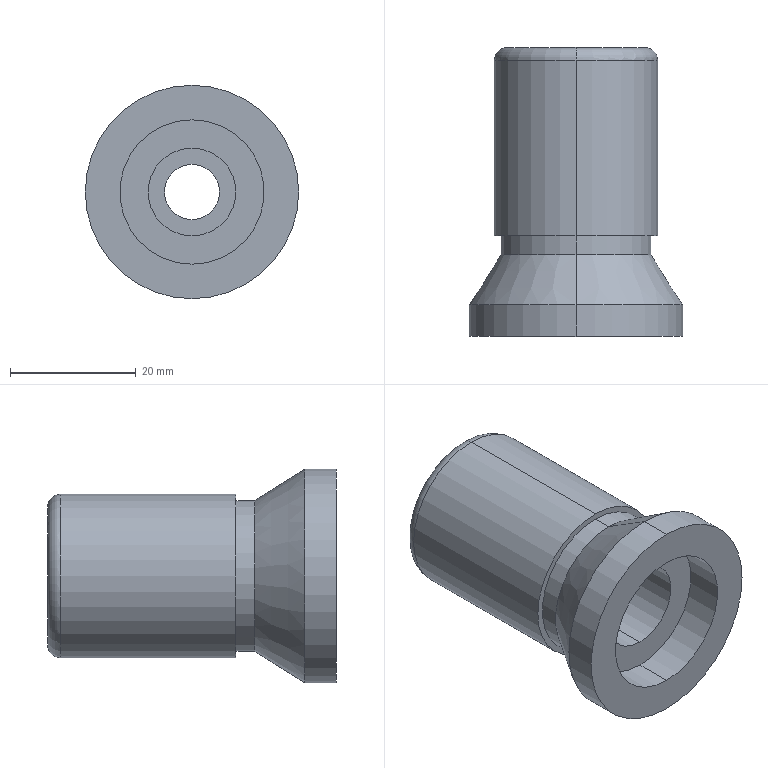Part | STEP file | 刮-墨刀压力镙母-1 | 1 solid | 21 faces | box 34 x 46 x 34 mm | volume 20305 mm3 | cylinder 12 | plane 5 | torus 2 | cone 2 | commonest cylinder face diameters 8.8 x2 14 x2 23 x2 24 x2 26 x2 34 x2
STEP:
#1=CARTESIAN_POINT('',(0.,0.,11.));
#2=VERTEX_POINT('',#1);
#3=CARTESIAN_POINT('',(0.,0.,-11.));
#4=VERTEX_POINT('',#3);
#5=CARTESIAN_POINT('',(0.,0.,0.));
#6=DIRECTION('',(0.,1.,0.));
#7=DIRECTION('',(0.,0.,-1.));
#8=AXIS2_PLACEMENT_3D('',#5,#6,#7);
#9=CIRCLE('',#8,11.);
#10=EDGE_CURVE('',#2,#4,#9,.T.);
#11=ORIENTED_EDGE('',*,*,#10,.F.);
#12=CARTESIAN_POINT('',(0.,-2.,13.));
#13=VERTEX_POINT('',#12);
#14=CARTESIAN_POINT('',(0.,-2.,11.));
#15=DIRECTION('',(1.,0.,0.));
#16=DIRECTION('',(0.,0.,-1.));
#17=AXIS2_PLACEMENT_3D('',#14,#15,#16);
#18=CIRCLE('',#17,2.);
#19=EDGE_CURVE('',#2,#13,#18,.T.);
#20=ORIENTED_EDGE('',*,*,#19,.T.);
#21=CARTESIAN_POINT('',(0.,-2.,-13.));
#22=VERTEX_POINT('',#21);
#23=CARTESIAN_POINT('',(0.,-2.,0.));
#24=DIRECTION('',(0.,-1.,0.));
#25=DIRECTION('',(0.,0.,-1.));
#26=AXIS2_PLACEMENT_3D('',#23,#24,#25);
#27=CIRCLE('',#26,13.);
#28=EDGE_CURVE('',#22,#13,#27,.T.);
#29=ORIENTED_EDGE('',*,*,#28,.F.);
#30=CARTESIAN_POINT('',(0.,-2.,-11.));
#31=DIRECTION('',(-1.,0.,0.));
#32=DIRECTION('',(0.,0.,1.));
#33=AXIS2_PLACEMENT_3D('',#30,#31,#32);
#34=CIRCLE('',#33,2.);
#35=EDGE_CURVE('',#4,#22,#34,.T.);
#36=ORIENTED_EDGE('',*,*,#35,.F.);
#37=EDGE_LOOP('',(#11,#20,#29,#36));
#38=FACE_OUTER_BOUND('',#37,.T.);
#39=CARTESIAN_POINT('',(0.,-2.,0.));
#40=DIRECTION('',(0.,-1.,0.));
#41=DIRECTION('',(0.,0.,-1.));
#42=AXIS2_PLACEMENT_3D('',#39,#40,#41);
#43=TOROIDAL_SURFACE('',#42,11.,2.);
#44=ADVANCED_FACE('',(#38),#43,.T.);
#45=CARTESIAN_POINT('',(0.,-20.,4.4));
#46=VERTEX_POINT('',#45);
#47=CARTESIAN_POINT('',(0.,-20.,-4.4));
#48=VERTEX_POINT('',#47);
#49=CARTESIAN_POINT('',(0.,-20.,0.));
#50=DIRECTION('',(0.,-1.,0.));
#51=DIRECTION('',(0.,0.,-1.));
#52=AXIS2_PLACEMENT_3D('',#49,#50,#51);
#53=CIRCLE('',#52,4.4);
#54=EDGE_CURVE('',#46,#48,#53,.T.);
#55=ORIENTED_EDGE('',*,*,#54,.T.);
#56=CARTESIAN_POINT('',(0.,0.,-4.4));
#57=VERTEX_POINT('',#56);
#58=CARTESIAN_POINT('',(0.,0.,-4.4));
#59=DIRECTION('',(0.,1.,0.));
#60=VECTOR('',#59,1000.);
#61=LINE('',#58,#60);
#62=EDGE_CURVE('',#48,#57,#61,.T.);
#63=ORIENTED_EDGE('',*,*,#62,.T.);
#64=CARTESIAN_POINT('',(0.,0.,4.4));
#65=VERTEX_POINT('',#64);
#66=CARTESIAN_POINT('',(0.,0.,0.));
#67=DIRECTION('',(0.,1.,0.));
#68=DIRECTION('',(0.,0.,1.));
#69=AXIS2_PLACEMENT_3D('',#66,#67,#68);
#70=CIRCLE('',#69,4.4);
#71=EDGE_CURVE('',#57,#65,#70,.T.);
#72=ORIENTED_EDGE('',*,*,#71,.T.);
#73=CARTESIAN_POINT('',(0.,0.,4.4));
#74=DIRECTION('',(0.,1.,0.));
#75=VECTOR('',#74,1000.);
#76=LINE('',#73,#75);
#77=EDGE_CURVE('',#46,#65,#76,.T.);
#78=ORIENTED_EDGE('',*,*,#77,.F.);
#79=EDGE_LOOP('',(#55,#63,#72,#78));
#80=FACE_OUTER_BOUND('',#79,.T.);
#81=CARTESIAN_POINT('',(0.,0.,0.));
#82=DIRECTION('',(0.,1.,0.));
#83=DIRECTION('',(0.,0.,1.));
#84=AXIS2_PLACEMENT_3D('',#81,#82,#83);
#85=CYLINDRICAL_SURFACE('',#84,4.4);
#86=ADVANCED_FACE('',(#80),#85,.F.);
#87=CARTESIAN_POINT('',(0.,-20.,7.));
#88=VERTEX_POINT('',#87);
#89=CARTESIAN_POINT('',(0.,-20.,-7.));
#90=VERTEX_POINT('',#89);
#91=CARTESIAN_POINT('',(0.,-20.,0.));
#92=DIRECTION('',(0.,-1.,0.));
#93=DIRECTION('',(0.,0.,-1.));
#94=AXIS2_PLACEMENT_3D('',#91,#92,#93);
#95=CIRCLE('',#94,7.);
#96=EDGE_CURVE('',#88,#90,#95,.T.);
#97=ORIENTED_EDGE('',*,*,#96,.F.);
#98=CARTESIAN_POINT('',(0.,-40.,7.));
#99=VERTEX_POINT('',#98);
#100=CARTESIAN_POINT('',(0.,-20.,7.));
#101=DIRECTION('',(0.,-1.,0.));
#102=VECTOR('',#101,1000.);
#103=LINE('',#100,#102);
#104=EDGE_CURVE('',#88,#99,#103,.T.);
#105=ORIENTED_EDGE('',*,*,#104,.T.);
#106=CARTESIAN_POINT('',(0.,-40.,-7.));
#107=VERTEX_POINT('',#106);
#108=CARTESIAN_POINT('',(0.,-40.,0.));
#109=DIRECTION('',(0.,-1.,0.));
#110=DIRECTION('',(0.,0.,-1.));
#111=AXIS2_PLACEMENT_3D('',#108,#109,#110);
#112=CIRCLE('',#111,7.);
#113=EDGE_CURVE('',#99,#107,#112,.T.);
#114=ORIENTED_EDGE('',*,*,#113,.T.);
#115=CARTESIAN_POINT('',(0.,-20.,-7.));
#116=DIRECTION('',(0.,-1.,0.));
#117=VECTOR('',#116,1000.);
#118=LINE('',#115,#117);
#119=EDGE_CURVE('',#90,#107,#118,.T.);
#120=ORIENTED_EDGE('',*,*,#119,.F.);
#121=EDGE_LOOP('',(#97,#105,#114,#120));
#122=FACE_OUTER_BOUND('',#121,.T.);
#123=CARTESIAN_POINT('',(0.,-20.,0.));
#124=DIRECTION('',(0.,-1.,0.));
#125=DIRECTION('',(0.,0.,-1.));
#126=AXIS2_PLACEMENT_3D('',#123,#124,#125);
#127=CYLINDRICAL_SURFACE('',#126,7.);
#128=ADVANCED_FACE('',(#122),#127,.F.);
#129=CARTESIAN_POINT('',(0.,-40.,11.5));
#130=VERTEX_POINT('',#129);
#131=CARTESIAN_POINT('',(0.,-40.,-11.5));
#132=VERTEX_POINT('',#131);
#133=CARTESIAN_POINT('',(0.,-40.,0.));
#134=DIRECTION('',(0.,-1.,0.));
#135=DIRECTION('',(0.,0.,-1.));
#136=AXIS2_PLACEMENT_3D('',#133,#134,#135);
#137=CIRCLE('',#136,11.5);
#138=EDGE_CURVE('',#130,#132,#137,.T.);
#139=ORIENTED_EDGE('',*,*,#138,.F.);
#140=CARTESIAN_POINT('',(0.,-46.,11.5));
#141=VERTEX_POINT('',#140);
#142=CARTESIAN_POINT('',(0.,-40.,11.5));
#143=DIRECTION('',(0.,-1.,0.));
#144=VECTOR('',#143,1000.);
#145=LINE('',#142,#144);
#146=EDGE_CURVE('',#130,#141,#145,.T.);
#147=ORIENTED_EDGE('',*,*,#146,.T.);
#148=CARTESIAN_POINT('',(0.,-46.,-11.5));
#149=VERTEX_POINT('',#148);
#150=CARTESIAN_POINT('',(0.,-46.,0.));
#151=DIRECTION('',(0.,-1.,0.));
#152=DIRECTION('',(0.,0.,-1.));
#153=AXIS2_PLACEMENT_3D('',#150,#151,#152);
#154=CIRCLE('',#153,11.5);
#155=EDGE_CURVE('',#141,#149,#154,.T.);
#156=ORIENTED_EDGE('',*,*,#155,.T.);
#157=CARTESIAN_POINT('',(0.,-40.,-11.5));
#158=DIRECTION('',(0.,-1.,0.));
#159=VECTOR('',#158,1000.);
#160=LINE('',#157,#159);
#161=EDGE_CURVE('',#132,#149,#160,.T.);
#162=ORIENTED_EDGE('',*,*,#161,.F.);
#163=EDGE_LOOP('',(#139,#147,#156,#162));
#164=FACE_OUTER_BOUND('',#163,.T.);
#165=CARTESIAN_POINT('',(0.,-40.,0.));
#166=DIRECTION('',(0.,-1.,0.));
#167=DIRECTION('',(0.,0.,-1.));
#168=AXIS2_PLACEMENT_3D('',#165,#166,#167);
#169=CYLINDRICAL_SURFACE('',#168,11.5);
#170=ADVANCED_FACE('',(#164),#169,.F.);
#171=CARTESIAN_POINT('',(0.,-46.,17.));
#172=VERTEX_POINT('',#171);
#173=CARTESIAN_POINT('',(0.,-46.,-17.));
#174=VERTEX_POINT('',#173);
#175=CARTESIAN_POINT('',(0.,-46.,0.));
#176=DIRECTION('',(0.,1.,0.));
#177=DIRECTION('',(0.,0.,1.));
#178=AXIS2_PLACEMENT_3D('',#175,#176,#177);
#179=CIRCLE('',#178,17.);
#180=EDGE_CURVE('',#172,#174,#179,.T.);
#181=ORIENTED_EDGE('',*,*,#180,.T.);
#182=CARTESIAN_POINT('',(0.,-41.,-17.));
#183=VERTEX_POINT('',#182);
#184=CARTESIAN_POINT('',(0.,0.,-17.));
#185=DIRECTION('',(0.,1.,0.));
#186=VECTOR('',#185,1000.);
#187=LINE('',#184,#186);
#188=EDGE_CURVE('',#174,#183,#187,.T.);
#189=ORIENTED_EDGE('',*,*,#188,.T.);
#190=CARTESIAN_POINT('',(0.,-41.,17.));
#191=VERTEX_POINT('',#190);
#192=CARTESIAN_POINT('',(0.,-41.,0.));
#193=DIRECTION('',(0.,1.,0.));
#194=DIRECTION('',(0.,0.,1.));
#195=AXIS2_PLACEMENT_3D('',#192,#193,#194);
#196=CIRCLE('',#195,17.);
#197=EDGE_CURVE('',#191,#183,#196,.T.);
#198=ORIENTED_EDGE('',*,*,#197,.F.);
#199=CARTESIAN_POINT('',(0.,0.,17.));
#200=DIRECTION('',(0.,1.,0.));
#201=VECTOR('',#200,1000.);
#202=LINE('',#199,#201);
#203=EDGE_CURVE('',#172,#191,#202,.T.);
#204=ORIENTED_EDGE('',*,*,#203,.F.);
#205=EDGE_LOOP('',(#181,#189,#198,#204));
#206=FACE_OUTER_BOUND('',#205,.T.);
#207=CARTESIAN_POINT('',(0.,0.,0.));
#208=DIRECTION('',(0.,1.,0.));
#209=DIRECTION('',(0.,0.,1.));
#210=AXIS2_PLACEMENT_3D('',#207,#208,#209);
#211=CYLINDRICAL_SURFACE('',#210,17.);
#212=ADVANCED_FACE('',(#206),#211,.T.);
#213=CARTESIAN_POINT('',(0.,-33.,12.));
#214=VERTEX_POINT('',#213);
#215=CARTESIAN_POINT('',(0.,-33.,-12.));
#216=VERTEX_POINT('',#215);
#217=CARTESIAN_POINT('',(0.,-33.,0.));
#218=DIRECTION('',(0.,1.,0.));
#219=DIRECTION('',(0.,0.,1.));
#220=AXIS2_PLACEMENT_3D('',#217,#218,#219);
#221=CIRCLE('',#220,12.);
#222=EDGE_CURVE('',#214,#216,#221,.T.);
#223=ORIENTED_EDGE('',*,*,#222,.F.);
#224=CARTESIAN_POINT('',(0.,-41.,17.));
#225=DIRECTION('',(0.,-0.848,0.53));
#226=VECTOR('',#225,1000.);
#227=LINE('',#224,#226);
#228=EDGE_CURVE('',#214,#191,#227,.T.);
#229=ORIENTED_EDGE('',*,*,#228,.T.);
#230=ORIENTED_EDGE('',*,*,#197,.T.);
#231=CARTESIAN_POINT('',(0.,-41.,-17.));
#232=DIRECTION('',(0.,-0.848,-0.53));
#233=VECTOR('',#232,1000.);
#234=LINE('',#231,#233);
#235=EDGE_CURVE('',#216,#183,#234,.T.);
#236=ORIENTED_EDGE('',*,*,#235,.F.);
#237=EDGE_LOOP('',(#223,#229,#230,#236));
#238=FACE_OUTER_BOUND('',#237,.T.);
#239=CARTESIAN_POINT('',(0.,-41.,0.));
#240=DIRECTION('',(0.,-1.,0.));
#241=DIRECTION('',(0.,0.,-1.));
#242=AXIS2_PLACEMENT_3D('',#239,#240,#241);
#243=CONICAL_SURFACE('',#242,17.,0.5586);
#244=ADVANCED_FACE('',(#238),#243,.T.);
#245=ORIENTED_EDGE('',*,*,#222,.T.);
#246=CARTESIAN_POINT('',(0.,-30.,-12.));
#247=VERTEX_POINT('',#246);
#248=CARTESIAN_POINT('',(0.,0.,-12.));
#249=DIRECTION('',(0.,1.,0.));
#250=VECTOR('',#249,1000.);
#251=LINE('',#248,#250);
#252=EDGE_CURVE('',#216,#247,#251,.T.);
#253=ORIENTED_EDGE('',*,*,#252,.T.);
#254=CARTESIAN_POINT('',(0.,-30.,12.));
#255=VERTEX_POINT('',#254);
#256=CARTESIAN_POINT('',(0.,-30.,0.));
#257=DIRECTION('',(0.,1.,0.));
#258=DIRECTION('',(0.,0.,1.));
#259=AXIS2_PLACEMENT_3D('',#256,#257,#258);
#260=CIRCLE('',#259,12.);
#261=EDGE_CURVE('',#255,#247,#260,.T.);
#262=ORIENTED_EDGE('',*,*,#261,.F.);
#263=CARTESIAN_POINT('',(0.,0.,12.));
#264=DIRECTION('',(0.,1.,0.));
#265=VECTOR('',#264,1000.);
#266=LINE('',#263,#265);
#267=EDGE_CURVE('',#214,#255,#266,.T.);
#268=ORIENTED_EDGE('',*,*,#267,.F.);
#269=EDGE_LOOP('',(#245,#253,#262,#268));
#270=FACE_OUTER_BOUND('',#269,.T.);
#271=CARTESIAN_POINT('',(0.,0.,0.));
#272=DIRECTION('',(0.,1.,0.));
#273=DIRECTION('',(0.,0.,1.));
#274=AXIS2_PLACEMENT_3D('',#271,#272,#273);
#275=CYLINDRICAL_SURFACE('',#274,12.);
#276=ADVANCED_FACE('',(#270),#275,.T.);
#277=CARTESIAN_POINT('',(0.,-30.,13.));
#278=VERTEX_POINT('',#277);
#279=CARTESIAN_POINT('',(0.,-30.,-13.));
#280=VERTEX_POINT('',#279);
#281=CARTESIAN_POINT('',(0.,-30.,0.));
#282=DIRECTION('',(0.,1.,0.));
#283=DIRECTION('',(0.,0.,1.));
#284=AXIS2_PLACEMENT_3D('',#281,#282,#283);
#285=CIRCLE('',#284,13.);
#286=EDGE_CURVE('',#278,#280,#285,.T.);
#287=ORIENTED_EDGE('',*,*,#286,.T.);
#288=CARTESIAN_POINT('',(0.,0.,-13.));
#289=DIRECTION('',(0.,1.,0.));
#290=VECTOR('',#289,1000.);
#291=LINE('',#288,#290);
#292=EDGE_CURVE('',#280,#22,#291,.T.);
#293=ORIENTED_EDGE('',*,*,#292,.T.);
#294=ORIENTED_EDGE('',*,*,#28,.T.);
#295=CARTESIAN_POINT('',(0.,0.,13.));
#296=DIRECTION('',(0.,1.,0.));
#297=VECTOR('',#296,1000.);
#298=LINE('',#295,#297);
#299=EDGE_CURVE('',#278,#13,#298,.T.);
#300=ORIENTED_EDGE('',*,*,#299,.F.);
#301=EDGE_LOOP('',(#287,#293,#294,#300));
#302=FACE_OUTER_BOUND('',#301,.T.);
#303=CARTESIAN_POINT('',(0.,0.,0.));
#304=DIRECTION('',(0.,1.,0.));
#305=DIRECTION('',(0.,0.,1.));
#306=AXIS2_PLACEMENT_3D('',#303,#304,#305);
#307=CYLINDRICAL_SURFACE('',#306,13.);
#308=ADVANCED_FACE('',(#302),#307,.T.);
#309=CARTESIAN_POINT('',(0.,0.,0.));
#310=DIRECTION('',(0.,1.,0.));
#311=DIRECTION('',(0.,0.,-1.));
#312=AXIS2_PLACEMENT_3D('',#309,#310,#311);
#313=CIRCLE('',#312,11.);
#314=EDGE_CURVE('',#4,#2,#313,.T.);
#315=ORIENTED_EDGE('',*,*,#314,.T.);
#316=ORIENTED_EDGE('',*,*,#10,.T.);
#317=EDGE_LOOP('',(#315,#316));
#318=FACE_OUTER_BOUND('',#317,.T.);
#319=CARTESIAN_POINT('',(0.,0.,0.));
#320=DIRECTION('',(0.,1.,0.));
#321=DIRECTION('',(0.,0.,1.));
#322=AXIS2_PLACEMENT_3D('',#319,#320,#321);
#323=CIRCLE('',#322,4.4);
#324=EDGE_CURVE('',#65,#57,#323,.T.);
#325=ORIENTED_EDGE('',*,*,#324,.F.);
#326=ORIENTED_EDGE('',*,*,#71,.F.);
#327=EDGE_LOOP('',(#325,#326));
#328=FACE_BOUND('',#327,.T.);
#329=CARTESIAN_POINT('',(0.,0.,0.));
#330=DIRECTION('',(0.,-1.,0.));
#331=DIRECTION('',(0.,0.,-1.));
#332=AXIS2_PLACEMENT_3D('',#329,#330,#331);
#333=PLANE('',#332);
#334=ADVANCED_FACE('',(#318,#328),#333,.F.);
#335=ORIENTED_EDGE('',*,*,#292,.F.);
#336=CARTESIAN_POINT('',(0.,-30.,0.));
#337=DIRECTION('',(0.,1.,0.));
#338=DIRECTION('',(0.,0.,1.));
#339=AXIS2_PLACEMENT_3D('',#336,#337,#338);
#340=CIRCLE('',#339,13.);
#341=EDGE_CURVE('',#280,#278,#340,.T.);
#342=ORIENTED_EDGE('',*,*,#341,.T.);
#343=ORIENTED_EDGE('',*,*,#299,.T.);
#344=CARTESIAN_POINT('',(0.,-2.,0.));
#345=DIRECTION('',(0.,-1.,0.));
#346=DIRECTION('',(0.,0.,-1.));
#347=AXIS2_PLACEMENT_3D('',#344,#345,#346);
#348=CIRCLE('',#347,13.);
#349=EDGE_CURVE('',#13,#22,#348,.T.);
#350=ORIENTED_EDGE('',*,*,#349,.T.);
#351=EDGE_LOOP('',(#335,#342,#343,#350));
#352=FACE_OUTER_BOUND('',#351,.T.);
#353=CARTESIAN_POINT('',(0.,0.,0.));
#354=DIRECTION('',(0.,1.,0.));
#355=DIRECTION('',(0.,0.,1.));
#356=AXIS2_PLACEMENT_3D('',#353,#354,#355);
#357=CYLINDRICAL_SURFACE('',#356,13.);
#358=ADVANCED_FACE('',(#352),#357,.T.);
#359=ORIENTED_EDGE('',*,*,#286,.F.);
#360=ORIENTED_EDGE('',*,*,#341,.F.);
#361=EDGE_LOOP('',(#359,#360));
#362=FACE_OUTER_BOUND('',#361,.T.);
#363=ORIENTED_EDGE('',*,*,#261,.T.);
#364=CARTESIAN_POINT('',(0.,-30.,0.));
#365=DIRECTION('',(0.,1.,0.));
#366=DIRECTION('',(0.,0.,1.));
#367=AXIS2_PLACEMENT_3D('',#364,#365,#366);
#368=CIRCLE('',#367,12.);
#369=EDGE_CURVE('',#247,#255,#368,.T.);
#370=ORIENTED_EDGE('',*,*,#369,.T.);
#371=EDGE_LOOP('',(#363,#370));
#372=FACE_BOUND('',#371,.T.);
#373=CARTESIAN_POINT('',(13.,-30.,0.));
#374=DIRECTION('',(0.,1.,0.));
#375=DIRECTION('',(0.,0.,1.));
#376=AXIS2_PLACEMENT_3D('',#373,#374,#375);
#377=PLANE('',#376);
#378=ADVANCED_FACE('',(#362,#372),#377,.F.);
#379=ORIENTED_EDGE('',*,*,#252,.F.);
#380=CARTESIAN_POINT('',(0.,-33.,0.));
#381=DIRECTION('',(0.,1.,0.));
#382=DIRECTION('',(0.,0.,1.));
#383=AXIS2_PLACEMENT_3D('',#380,#381,#382);
#384=CIRCLE('',#383,12.);
#385=EDGE_CURVE('',#216,#214,#384,.T.);
#386=ORIENTED_EDGE('',*,*,#385,.T.);
#387=ORIENTED_EDGE('',*,*,#267,.T.);
#388=ORIENTED_EDGE('',*,*,#369,.F.);
#389=EDGE_LOOP('',(#379,#386,#387,#388));
#390=FACE_OUTER_BOUND('',#389,.T.);
#391=CARTESIAN_POINT('',(0.,0.,0.));
#392=DIRECTION('',(0.,1.,0.));
#393=DIRECTION('',(0.,0.,1.));
#394=AXIS2_PLACEMENT_3D('',#391,#392,#393);
#395=CYLINDRICAL_SURFACE('',#394,12.);
#396=ADVANCED_FACE('',(#390),#395,.T.);
#397=ORIENTED_EDGE('',*,*,#228,.F.);
#398=ORIENTED_EDGE('',*,*,#385,.F.);
#399=ORIENTED_EDGE('',*,*,#235,.T.);
#400=CARTESIAN_POINT('',(0.,-41.,0.));
#401=DIRECTION('',(0.,1.,0.));
#402=DIRECTION('',(0.,0.,1.));
#403=AXIS2_PLACEMENT_3D('',#400,#401,#402);
#404=CIRCLE('',#403,17.);
#405=EDGE_CURVE('',#183,#191,#404,.T.);
#406=ORIENTED_EDGE('',*,*,#405,.T.);
#407=EDGE_LOOP('',(#397,#398,#399,#406));
#408=FACE_OUTER_BOUND('',#407,.T.);
#409=CARTESIAN_POINT('',(0.,-41.,0.));
#410=DIRECTION('',(0.,-1.,0.));
#411=DIRECTION('',(0.,0.,-1.));
#412=AXIS2_PLACEMENT_3D('',#409,#410,#411);
#413=CONICAL_SURFACE('',#412,17.,0.5586);
#414=ADVANCED_FACE('',(#408),#413,.T.);
#415=ORIENTED_EDGE('',*,*,#188,.F.);
#416=CARTESIAN_POINT('',(0.,-46.,0.));
#417=DIRECTION('',(0.,1.,0.));
#418=DIRECTION('',(0.,0.,1.));
#419=AXIS2_PLACEMENT_3D('',#416,#417,#418);
#420=CIRCLE('',#419,17.);
#421=EDGE_CURVE('',#174,#172,#420,.T.);
#422=ORIENTED_EDGE('',*,*,#421,.T.);
#423=ORIENTED_EDGE('',*,*,#203,.T.);
#424=ORIENTED_EDGE('',*,*,#405,.F.);
#425=EDGE_LOOP('',(#415,#422,#423,#424));
#426=FACE_OUTER_BOUND('',#425,.T.);
#427=CARTESIAN_POINT('',(0.,0.,0.));
#428=DIRECTION('',(0.,1.,0.));
#429=DIRECTION('',(0.,0.,1.));
#430=AXIS2_PLACEMENT_3D('',#427,#428,#429);
#431=CYLINDRICAL_SURFACE('',#430,17.);
#432=ADVANCED_FACE('',(#426),#431,.T.);
#433=CARTESIAN_POINT('',(0.,-46.,0.));
#434=DIRECTION('',(0.,-1.,0.));
#435=DIRECTION('',(0.,0.,-1.));
#436=AXIS2_PLACEMENT_3D('',#433,#434,#435);
#437=CIRCLE('',#436,11.5);
#438=EDGE_CURVE('',#149,#141,#437,.T.);
#439=ORIENTED_EDGE('',*,*,#438,.F.);
#440=ORIENTED_EDGE('',*,*,#155,.F.);
#441=EDGE_LOOP('',(#439,#440));
#442=FACE_BOUND('',#441,.T.);
#443=ORIENTED_EDGE('',*,*,#180,.F.);
#444=ORIENTED_EDGE('',*,*,#421,.F.);
#445=EDGE_LOOP('',(#443,#444));
#446=FACE_OUTER_BOUND('',#445,.T.);
#447=CARTESIAN_POINT('',(17.,-46.,0.));
#448=DIRECTION('',(0.,1.,0.));
#449=DIRECTION('',(0.,0.,1.));
#450=AXIS2_PLACEMENT_3D('',#447,#448,#449);
#451=PLANE('',#450);
#452=ADVANCED_FACE('',(#442,#446),#451,.F.);
#453=ORIENTED_EDGE('',*,*,#146,.F.);
#454=CARTESIAN_POINT('',(0.,-40.,0.));
#455=DIRECTION('',(0.,-1.,0.));
#456=DIRECTION('',(0.,0.,-1.));
#457=AXIS2_PLACEMENT_3D('',#454,#455,#456);
#458=CIRCLE('',#457,11.5);
#459=EDGE_CURVE('',#132,#130,#458,.T.);
#460=ORIENTED_EDGE('',*,*,#459,.F.);
#461=ORIENTED_EDGE('',*,*,#161,.T.);
#462=ORIENTED_EDGE('',*,*,#438,.T.);
#463=EDGE_LOOP('',(#453,#460,#461,#462));
#464=FACE_OUTER_BOUND('',#463,.T.);
#465=CARTESIAN_POINT('',(0.,-40.,0.));
#466=DIRECTION('',(0.,-1.,0.));
#467=DIRECTION('',(0.,0.,-1.));
#468=AXIS2_PLACEMENT_3D('',#465,#466,#467);
#469=CYLINDRICAL_SURFACE('',#468,11.5);
#470=ADVANCED_FACE('',(#464),#469,.F.);
#471=CARTESIAN_POINT('',(0.,-40.,0.));
#472=DIRECTION('',(0.,-1.,0.));
#473=DIRECTION('',(0.,0.,-1.));
#474=AXIS2_PLACEMENT_3D('',#471,#472,#473);
#475=CIRCLE('',#474,7.);
#476=EDGE_CURVE('',#107,#99,#475,.T.);
#477=ORIENTED_EDGE('',*,*,#476,.F.);
#478=ORIENTED_EDGE('',*,*,#113,.F.);
#479=EDGE_LOOP('',(#477,#478));
#480=FACE_BOUND('',#479,.T.);
#481=ORIENTED_EDGE('',*,*,#459,.T.);
#482=ORIENTED_EDGE('',*,*,#138,.T.);
#483=EDGE_LOOP('',(#481,#482));
#484=FACE_OUTER_BOUND('',#483,.T.);
#485=CARTESIAN_POINT('',(0.,-40.,0.));
#486=DIRECTION('',(0.,-1.,0.));
#487=DIRECTION('',(0.,0.,-1.));
#488=AXIS2_PLACEMENT_3D('',#485,#486,#487);
#489=PLANE('',#488);
#490=ADVANCED_FACE('',(#480,#484),#489,.T.);
#491=ORIENTED_EDGE('',*,*,#104,.F.);
#492=CARTESIAN_POINT('',(0.,-20.,0.));
#493=DIRECTION('',(0.,-1.,0.));
#494=DIRECTION('',(0.,0.,-1.));
#495=AXIS2_PLACEMENT_3D('',#492,#493,#494);
#496=CIRCLE('',#495,7.);
#497=EDGE_CURVE('',#90,#88,#496,.T.);
#498=ORIENTED_EDGE('',*,*,#497,.F.);
#499=ORIENTED_EDGE('',*,*,#119,.T.);
#500=ORIENTED_EDGE('',*,*,#476,.T.);
#501=EDGE_LOOP('',(#491,#498,#499,#500));
#502=FACE_OUTER_BOUND('',#501,.T.);
#503=CARTESIAN_POINT('',(0.,-20.,0.));
#504=DIRECTION('',(0.,-1.,0.));
#505=DIRECTION('',(0.,0.,-1.));
#506=AXIS2_PLACEMENT_3D('',#503,#504,#505);
#507=CYLINDRICAL_SURFACE('',#506,7.);
#508=ADVANCED_FACE('',(#502),#507,.F.);
#509=ORIENTED_EDGE('',*,*,#54,.F.);
#510=CARTESIAN_POINT('',(0.,-20.,0.));
#511=DIRECTION('',(0.,-1.,0.));
#512=DIRECTION('',(0.,0.,-1.));
#513=AXIS2_PLACEMENT_3D('',#510,#511,#512);
#514=CIRCLE('',#513,4.4);
#515=EDGE_CURVE('',#48,#46,#514,.T.);
#516=ORIENTED_EDGE('',*,*,#515,.F.);
#517=EDGE_LOOP('',(#509,#516));
#518=FACE_BOUND('',#517,.T.);
#519=ORIENTED_EDGE('',*,*,#497,.T.);
#520=ORIENTED_EDGE('',*,*,#96,.T.);
#521=EDGE_LOOP('',(#519,#520));
#522=FACE_OUTER_BOUND('',#521,.T.);
#523=CARTESIAN_POINT('',(0.,-20.,0.));
#524=DIRECTION('',(0.,-1.,0.));
#525=DIRECTION('',(0.,0.,-1.));
#526=AXIS2_PLACEMENT_3D('',#523,#524,#525);
#527=PLANE('',#526);
#528=ADVANCED_FACE('',(#518,#522),#527,.T.);
#529=ORIENTED_EDGE('',*,*,#62,.F.);
#530=ORIENTED_EDGE('',*,*,#515,.T.);
#531=ORIENTED_EDGE('',*,*,#77,.T.);
#532=ORIENTED_EDGE('',*,*,#324,.T.);
#533=EDGE_LOOP('',(#529,#530,#531,#532));
#534=FACE_OUTER_BOUND('',#533,.T.);
#535=CARTESIAN_POINT('',(0.,0.,0.));
#536=DIRECTION('',(0.,1.,0.));
#537=DIRECTION('',(0.,0.,1.));
#538=AXIS2_PLACEMENT_3D('',#535,#536,#537);
#539=CYLINDRICAL_SURFACE('',#538,4.4);
#540=ADVANCED_FACE('',(#534),#539,.F.);
#541=ORIENTED_EDGE('',*,*,#19,.F.);
#542=ORIENTED_EDGE('',*,*,#314,.F.);
#543=ORIENTED_EDGE('',*,*,#35,.T.);
#544=ORIENTED_EDGE('',*,*,#349,.F.);
#545=EDGE_LOOP('',(#541,#542,#543,#544));
#546=FACE_OUTER_BOUND('',#545,.T.);
#547=CARTESIAN_POINT('',(0.,-2.,0.));
#548=DIRECTION('',(0.,-1.,0.));
#549=DIRECTION('',(0.,0.,-1.));
#550=AXIS2_PLACEMENT_3D('',#547,#548,#549);
#551=TOROIDAL_SURFACE('',#550,11.,2.);
#552=ADVANCED_FACE('',(#546),#551,.T.);
#553=CLOSED_SHELL('',(#44,#86,#128,#170,#212,#244,#276,#308,#334,#358,#378,#396,#414,#432,#452,#470,#490,#508,#528,#540,#552));
#554=MANIFOLD_SOLID_BREP('',#553);
#555=CARTESIAN_POINT('',(0.,0.,0.));
#556=DIRECTION('',(0.,0.,1.));
#557=DIRECTION('',(1.,0.,0.));
#558=AXIS2_PLACEMENT_3D('',#555,#556,#557);
#559=(LENGTH_UNIT()NAMED_UNIT(*)SI_UNIT(.MILLI.,.METRE.));
#560=UNCERTAINTY_MEASURE_WITH_UNIT(LENGTH_MEASURE(0.00001),#559,'','');
#561=(NAMED_UNIT(*)PLANE_ANGLE_UNIT()SI_UNIT($,.RADIAN.));
#562=(NAMED_UNIT(*)SI_UNIT($,.STERADIAN.)SOLID_ANGLE_UNIT());
#563=(GEOMETRIC_REPRESENTATION_CONTEXT(3)GLOBAL_UNCERTAINTY_ASSIGNED_CONTEXT((#560))GLOBAL_UNIT_ASSIGNED_CONTEXT((#559,#561,#562))REPRESENTATION_CONTEXT('',''));
#564=ADVANCED_BREP_SHAPE_REPRESENTATION('',(#554,#558),#563);